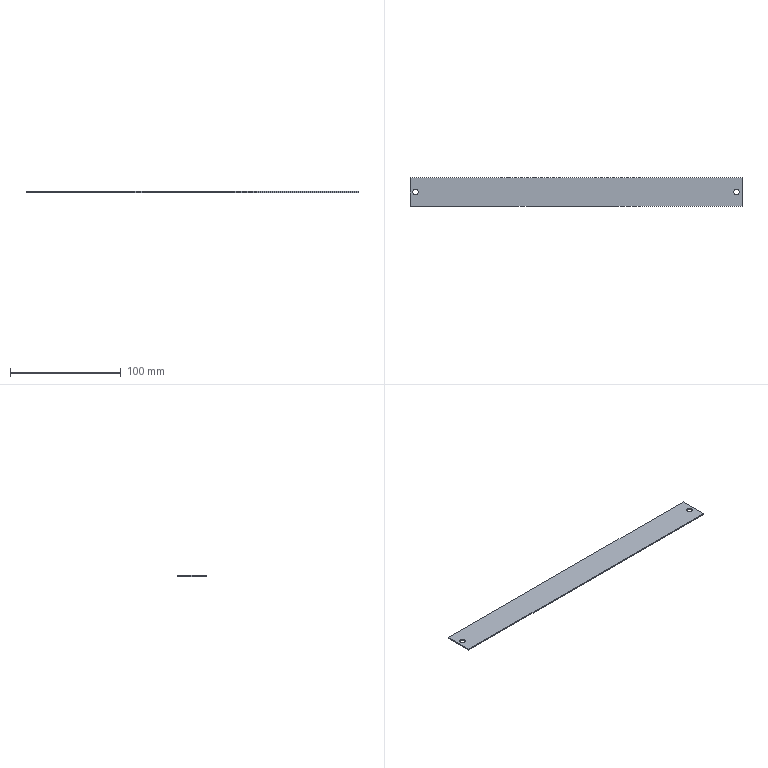Part | SolidWorks | features Extrusion 1, HoleWzd 1 | 1 solid | 10 faces | box 300 x 26 x 1 mm | volume 7761 mm3 | plane 6 | cylinder 4 | commonest cylinder face diameters 5 x4
STEP:
#1=CARTESIAN_POINT('',(-147.5,13.,0.));
#2=VERTEX_POINT('',#1);
#3=CARTESIAN_POINT('',(-142.5,13.,0.));
#4=VERTEX_POINT('',#3);
#5=CARTESIAN_POINT('',(-145.,13.,0.));
#6=DIRECTION('',(0.,0.,1.));
#7=DIRECTION('',(1.,0.,0.));
#8=AXIS2_PLACEMENT_3D('',#5,#6,#7);
#9=CIRCLE('',#8,2.5);
#10=EDGE_CURVE('',#2,#4,#9,.T.);
#11=ORIENTED_EDGE('',*,*,#10,.F.);
#12=CARTESIAN_POINT('',(-147.5,13.,1.));
#13=VERTEX_POINT('',#12);
#14=CARTESIAN_POINT('',(-147.5,13.,1.));
#15=DIRECTION('',(0.,0.,1.));
#16=VECTOR('',#15,1000.);
#17=LINE('',#14,#16);
#18=EDGE_CURVE('',#2,#13,#17,.T.);
#19=ORIENTED_EDGE('',*,*,#18,.T.);
#20=CARTESIAN_POINT('',(-142.5,13.,1.));
#21=VERTEX_POINT('',#20);
#22=CARTESIAN_POINT('',(-145.,13.,1.));
#23=DIRECTION('',(0.,0.,1.));
#24=DIRECTION('',(1.,0.,0.));
#25=AXIS2_PLACEMENT_3D('',#22,#23,#24);
#26=CIRCLE('',#25,2.5);
#27=EDGE_CURVE('',#13,#21,#26,.T.);
#28=ORIENTED_EDGE('',*,*,#27,.T.);
#29=CARTESIAN_POINT('',(-142.5,13.,1.));
#30=DIRECTION('',(0.,0.,1.));
#31=VECTOR('',#30,1000.);
#32=LINE('',#29,#31);
#33=EDGE_CURVE('',#4,#21,#32,.T.);
#34=ORIENTED_EDGE('',*,*,#33,.F.);
#35=EDGE_LOOP('',(#11,#19,#28,#34));
#36=FACE_OUTER_BOUND('',#35,.T.);
#37=CARTESIAN_POINT('',(-145.,13.,1.));
#38=DIRECTION('',(0.,0.,1.));
#39=DIRECTION('',(1.,0.,0.));
#40=AXIS2_PLACEMENT_3D('',#37,#38,#39);
#41=CYLINDRICAL_SURFACE('',#40,2.5);
#42=ADVANCED_FACE('',(#36),#41,.F.);
#43=CARTESIAN_POINT('',(142.5,13.,0.));
#44=VERTEX_POINT('',#43);
#45=CARTESIAN_POINT('',(147.5,13.,0.));
#46=VERTEX_POINT('',#45);
#47=CARTESIAN_POINT('',(145.,13.,0.));
#48=DIRECTION('',(0.,0.,1.));
#49=DIRECTION('',(1.,0.,0.));
#50=AXIS2_PLACEMENT_3D('',#47,#48,#49);
#51=CIRCLE('',#50,2.5);
#52=EDGE_CURVE('',#44,#46,#51,.T.);
#53=ORIENTED_EDGE('',*,*,#52,.F.);
#54=CARTESIAN_POINT('',(142.5,13.,1.));
#55=VERTEX_POINT('',#54);
#56=CARTESIAN_POINT('',(142.5,13.,1.));
#57=DIRECTION('',(0.,0.,1.));
#58=VECTOR('',#57,1000.);
#59=LINE('',#56,#58);
#60=EDGE_CURVE('',#44,#55,#59,.T.);
#61=ORIENTED_EDGE('',*,*,#60,.T.);
#62=CARTESIAN_POINT('',(147.5,13.,1.));
#63=VERTEX_POINT('',#62);
#64=CARTESIAN_POINT('',(145.,13.,1.));
#65=DIRECTION('',(0.,0.,1.));
#66=DIRECTION('',(1.,0.,0.));
#67=AXIS2_PLACEMENT_3D('',#64,#65,#66);
#68=CIRCLE('',#67,2.5);
#69=EDGE_CURVE('',#55,#63,#68,.T.);
#70=ORIENTED_EDGE('',*,*,#69,.T.);
#71=CARTESIAN_POINT('',(147.5,13.,1.));
#72=DIRECTION('',(0.,0.,1.));
#73=VECTOR('',#72,1000.);
#74=LINE('',#71,#73);
#75=EDGE_CURVE('',#46,#63,#74,.T.);
#76=ORIENTED_EDGE('',*,*,#75,.F.);
#77=EDGE_LOOP('',(#53,#61,#70,#76));
#78=FACE_OUTER_BOUND('',#77,.T.);
#79=CARTESIAN_POINT('',(145.,13.,1.));
#80=DIRECTION('',(0.,0.,1.));
#81=DIRECTION('',(1.,0.,0.));
#82=AXIS2_PLACEMENT_3D('',#79,#80,#81);
#83=CYLINDRICAL_SURFACE('',#82,2.5);
#84=ADVANCED_FACE('',(#78),#83,.F.);
#85=CARTESIAN_POINT('',(-150.,26.,0.));
#86=VERTEX_POINT('',#85);
#87=CARTESIAN_POINT('',(-150.,0.,0.));
#88=VERTEX_POINT('',#87);
#89=CARTESIAN_POINT('',(-150.,26.,0.));
#90=DIRECTION('',(0.,-1.,0.));
#91=VECTOR('',#90,1000.);
#92=LINE('',#89,#91);
#93=EDGE_CURVE('',#86,#88,#92,.T.);
#94=ORIENTED_EDGE('',*,*,#93,.T.);
#95=CARTESIAN_POINT('',(-150.,0.,1.));
#96=VERTEX_POINT('',#95);
#97=CARTESIAN_POINT('',(-150.,0.,1.));
#98=DIRECTION('',(0.,0.,-1.));
#99=VECTOR('',#98,1000.);
#100=LINE('',#97,#99);
#101=EDGE_CURVE('',#96,#88,#100,.T.);
#102=ORIENTED_EDGE('',*,*,#101,.F.);
#103=CARTESIAN_POINT('',(-150.,26.,1.));
#104=VERTEX_POINT('',#103);
#105=CARTESIAN_POINT('',(-150.,26.,1.));
#106=DIRECTION('',(0.,-1.,0.));
#107=VECTOR('',#106,1000.);
#108=LINE('',#105,#107);
#109=EDGE_CURVE('',#104,#96,#108,.T.);
#110=ORIENTED_EDGE('',*,*,#109,.F.);
#111=CARTESIAN_POINT('',(-150.,26.,1.));
#112=DIRECTION('',(0.,0.,-1.));
#113=VECTOR('',#112,1000.);
#114=LINE('',#111,#113);
#115=EDGE_CURVE('',#104,#86,#114,.T.);
#116=ORIENTED_EDGE('',*,*,#115,.T.);
#117=EDGE_LOOP('',(#94,#102,#110,#116));
#118=FACE_OUTER_BOUND('',#117,.T.);
#119=CARTESIAN_POINT('',(-150.,26.,1.));
#120=DIRECTION('',(1.,0.,0.));
#121=DIRECTION('',(0.,1.,0.));
#122=AXIS2_PLACEMENT_3D('',#119,#120,#121);
#123=PLANE('',#122);
#124=ADVANCED_FACE('',(#118),#123,.F.);
#125=CARTESIAN_POINT('',(150.,0.,0.));
#126=VERTEX_POINT('',#125);
#127=CARTESIAN_POINT('',(-150.,0.,0.));
#128=DIRECTION('',(1.,0.,0.));
#129=VECTOR('',#128,1000.);
#130=LINE('',#127,#129);
#131=EDGE_CURVE('',#88,#126,#130,.T.);
#132=ORIENTED_EDGE('',*,*,#131,.T.);
#133=CARTESIAN_POINT('',(150.,0.,1.));
#134=VERTEX_POINT('',#133);
#135=CARTESIAN_POINT('',(150.,0.,1.));
#136=DIRECTION('',(0.,0.,-1.));
#137=VECTOR('',#136,1000.);
#138=LINE('',#135,#137);
#139=EDGE_CURVE('',#134,#126,#138,.T.);
#140=ORIENTED_EDGE('',*,*,#139,.F.);
#141=CARTESIAN_POINT('',(-150.,0.,1.));
#142=DIRECTION('',(1.,0.,0.));
#143=VECTOR('',#142,1000.);
#144=LINE('',#141,#143);
#145=EDGE_CURVE('',#96,#134,#144,.T.);
#146=ORIENTED_EDGE('',*,*,#145,.F.);
#147=ORIENTED_EDGE('',*,*,#101,.T.);
#148=EDGE_LOOP('',(#132,#140,#146,#147));
#149=FACE_OUTER_BOUND('',#148,.T.);
#150=CARTESIAN_POINT('',(-150.,0.,1.));
#151=DIRECTION('',(0.,1.,0.));
#152=DIRECTION('',(0.,0.,1.));
#153=AXIS2_PLACEMENT_3D('',#150,#151,#152);
#154=PLANE('',#153);
#155=ADVANCED_FACE('',(#149),#154,.F.);
#156=CARTESIAN_POINT('',(150.,26.,0.));
#157=VERTEX_POINT('',#156);
#158=CARTESIAN_POINT('',(150.,26.,0.));
#159=DIRECTION('',(0.,1.,0.));
#160=VECTOR('',#159,1000.);
#161=LINE('',#158,#160);
#162=EDGE_CURVE('',#126,#157,#161,.T.);
#163=ORIENTED_EDGE('',*,*,#162,.T.);
#164=CARTESIAN_POINT('',(150.,26.,1.));
#165=VERTEX_POINT('',#164);
#166=CARTESIAN_POINT('',(150.,26.,1.));
#167=DIRECTION('',(0.,0.,-1.));
#168=VECTOR('',#167,1000.);
#169=LINE('',#166,#168);
#170=EDGE_CURVE('',#165,#157,#169,.T.);
#171=ORIENTED_EDGE('',*,*,#170,.F.);
#172=CARTESIAN_POINT('',(150.,26.,1.));
#173=DIRECTION('',(0.,1.,0.));
#174=VECTOR('',#173,1000.);
#175=LINE('',#172,#174);
#176=EDGE_CURVE('',#134,#165,#175,.T.);
#177=ORIENTED_EDGE('',*,*,#176,.F.);
#178=ORIENTED_EDGE('',*,*,#139,.T.);
#179=EDGE_LOOP('',(#163,#171,#177,#178));
#180=FACE_OUTER_BOUND('',#179,.T.);
#181=CARTESIAN_POINT('',(150.,26.,1.));
#182=DIRECTION('',(-1.,0.,0.));
#183=DIRECTION('',(0.,-1.,0.));
#184=AXIS2_PLACEMENT_3D('',#181,#182,#183);
#185=PLANE('',#184);
#186=ADVANCED_FACE('',(#180),#185,.F.);
#187=CARTESIAN_POINT('',(-150.,26.,0.));
#188=DIRECTION('',(-1.,0.,0.));
#189=VECTOR('',#188,1000.);
#190=LINE('',#187,#189);
#191=EDGE_CURVE('',#157,#86,#190,.T.);
#192=ORIENTED_EDGE('',*,*,#191,.T.);
#193=ORIENTED_EDGE('',*,*,#115,.F.);
#194=CARTESIAN_POINT('',(-150.,26.,1.));
#195=DIRECTION('',(-1.,0.,0.));
#196=VECTOR('',#195,1000.);
#197=LINE('',#194,#196);
#198=EDGE_CURVE('',#165,#104,#197,.T.);
#199=ORIENTED_EDGE('',*,*,#198,.F.);
#200=ORIENTED_EDGE('',*,*,#170,.T.);
#201=EDGE_LOOP('',(#192,#193,#199,#200));
#202=FACE_OUTER_BOUND('',#201,.T.);
#203=CARTESIAN_POINT('',(-150.,26.,1.));
#204=DIRECTION('',(0.,-1.,0.));
#205=DIRECTION('',(0.,0.,-1.));
#206=AXIS2_PLACEMENT_3D('',#203,#204,#205);
#207=PLANE('',#206);
#208=ADVANCED_FACE('',(#202),#207,.F.);
#209=CARTESIAN_POINT('',(-145.,13.,1.));
#210=DIRECTION('',(0.,0.,1.));
#211=DIRECTION('',(1.,0.,0.));
#212=AXIS2_PLACEMENT_3D('',#209,#210,#211);
#213=CIRCLE('',#212,2.5);
#214=EDGE_CURVE('',#21,#13,#213,.T.);
#215=ORIENTED_EDGE('',*,*,#214,.F.);
#216=ORIENTED_EDGE('',*,*,#27,.F.);
#217=EDGE_LOOP('',(#215,#216));
#218=FACE_BOUND('',#217,.T.);
#219=CARTESIAN_POINT('',(145.,13.,1.));
#220=DIRECTION('',(0.,0.,1.));
#221=DIRECTION('',(1.,0.,0.));
#222=AXIS2_PLACEMENT_3D('',#219,#220,#221);
#223=CIRCLE('',#222,2.5);
#224=EDGE_CURVE('',#63,#55,#223,.T.);
#225=ORIENTED_EDGE('',*,*,#224,.F.);
#226=ORIENTED_EDGE('',*,*,#69,.F.);
#227=EDGE_LOOP('',(#225,#226));
#228=FACE_BOUND('',#227,.T.);
#229=ORIENTED_EDGE('',*,*,#109,.T.);
#230=ORIENTED_EDGE('',*,*,#145,.T.);
#231=ORIENTED_EDGE('',*,*,#176,.T.);
#232=ORIENTED_EDGE('',*,*,#198,.T.);
#233=EDGE_LOOP('',(#229,#230,#231,#232));
#234=FACE_OUTER_BOUND('',#233,.T.);
#235=CARTESIAN_POINT('',(0.,0.,1.));
#236=DIRECTION('',(0.,0.,1.));
#237=DIRECTION('',(1.,0.,0.));
#238=AXIS2_PLACEMENT_3D('',#235,#236,#237);
#239=PLANE('',#238);
#240=ADVANCED_FACE('',(#218,#228,#234),#239,.T.);
#241=CARTESIAN_POINT('',(-145.,13.,0.));
#242=DIRECTION('',(0.,0.,1.));
#243=DIRECTION('',(1.,0.,0.));
#244=AXIS2_PLACEMENT_3D('',#241,#242,#243);
#245=CIRCLE('',#244,2.5);
#246=EDGE_CURVE('',#4,#2,#245,.T.);
#247=ORIENTED_EDGE('',*,*,#246,.T.);
#248=ORIENTED_EDGE('',*,*,#10,.T.);
#249=EDGE_LOOP('',(#247,#248));
#250=FACE_BOUND('',#249,.T.);
#251=CARTESIAN_POINT('',(145.,13.,0.));
#252=DIRECTION('',(0.,0.,1.));
#253=DIRECTION('',(1.,0.,0.));
#254=AXIS2_PLACEMENT_3D('',#251,#252,#253);
#255=CIRCLE('',#254,2.5);
#256=EDGE_CURVE('',#46,#44,#255,.T.);
#257=ORIENTED_EDGE('',*,*,#256,.T.);
#258=ORIENTED_EDGE('',*,*,#52,.T.);
#259=EDGE_LOOP('',(#257,#258));
#260=FACE_BOUND('',#259,.T.);
#261=ORIENTED_EDGE('',*,*,#93,.F.);
#262=ORIENTED_EDGE('',*,*,#191,.F.);
#263=ORIENTED_EDGE('',*,*,#162,.F.);
#264=ORIENTED_EDGE('',*,*,#131,.F.);
#265=EDGE_LOOP('',(#261,#262,#263,#264));
#266=FACE_OUTER_BOUND('',#265,.T.);
#267=CARTESIAN_POINT('',(0.,0.,0.));
#268=DIRECTION('',(0.,0.,1.));
#269=DIRECTION('',(1.,0.,0.));
#270=AXIS2_PLACEMENT_3D('',#267,#268,#269);
#271=PLANE('',#270);
#272=ADVANCED_FACE('',(#250,#260,#266),#271,.F.);
#273=ORIENTED_EDGE('',*,*,#60,.F.);
#274=ORIENTED_EDGE('',*,*,#256,.F.);
#275=ORIENTED_EDGE('',*,*,#75,.T.);
#276=ORIENTED_EDGE('',*,*,#224,.T.);
#277=EDGE_LOOP('',(#273,#274,#275,#276));
#278=FACE_OUTER_BOUND('',#277,.T.);
#279=CARTESIAN_POINT('',(145.,13.,1.));
#280=DIRECTION('',(0.,0.,1.));
#281=DIRECTION('',(1.,0.,0.));
#282=AXIS2_PLACEMENT_3D('',#279,#280,#281);
#283=CYLINDRICAL_SURFACE('',#282,2.5);
#284=ADVANCED_FACE('',(#278),#283,.F.);
#285=ORIENTED_EDGE('',*,*,#18,.F.);
#286=ORIENTED_EDGE('',*,*,#246,.F.);
#287=ORIENTED_EDGE('',*,*,#33,.T.);
#288=ORIENTED_EDGE('',*,*,#214,.T.);
#289=EDGE_LOOP('',(#285,#286,#287,#288));
#290=FACE_OUTER_BOUND('',#289,.T.);
#291=CARTESIAN_POINT('',(-145.,13.,1.));
#292=DIRECTION('',(0.,0.,1.));
#293=DIRECTION('',(1.,0.,0.));
#294=AXIS2_PLACEMENT_3D('',#291,#292,#293);
#295=CYLINDRICAL_SURFACE('',#294,2.5);
#296=ADVANCED_FACE('',(#290),#295,.F.);
#297=CLOSED_SHELL('',(#42,#84,#124,#155,#186,#208,#240,#272,#284,#296));
#298=MANIFOLD_SOLID_BREP('',#297);
#299=CARTESIAN_POINT('',(0.,0.,0.));
#300=DIRECTION('',(0.,0.,1.));
#301=DIRECTION('',(1.,0.,0.));
#302=AXIS2_PLACEMENT_3D('',#299,#300,#301);
#303=(LENGTH_UNIT()NAMED_UNIT(*)SI_UNIT(.MILLI.,.METRE.));
#304=UNCERTAINTY_MEASURE_WITH_UNIT(LENGTH_MEASURE(0.00001),#303,'','');
#305=(NAMED_UNIT(*)PLANE_ANGLE_UNIT()SI_UNIT($,.RADIAN.));
#306=(NAMED_UNIT(*)SI_UNIT($,.STERADIAN.)SOLID_ANGLE_UNIT());
#307=(GEOMETRIC_REPRESENTATION_CONTEXT(3)GLOBAL_UNCERTAINTY_ASSIGNED_CONTEXT((#304))GLOBAL_UNIT_ASSIGNED_CONTEXT((#303,#305,#306))REPRESENTATION_CONTEXT('',''));
#308=ADVANCED_BREP_SHAPE_REPRESENTATION('',(#298,#302),#307);